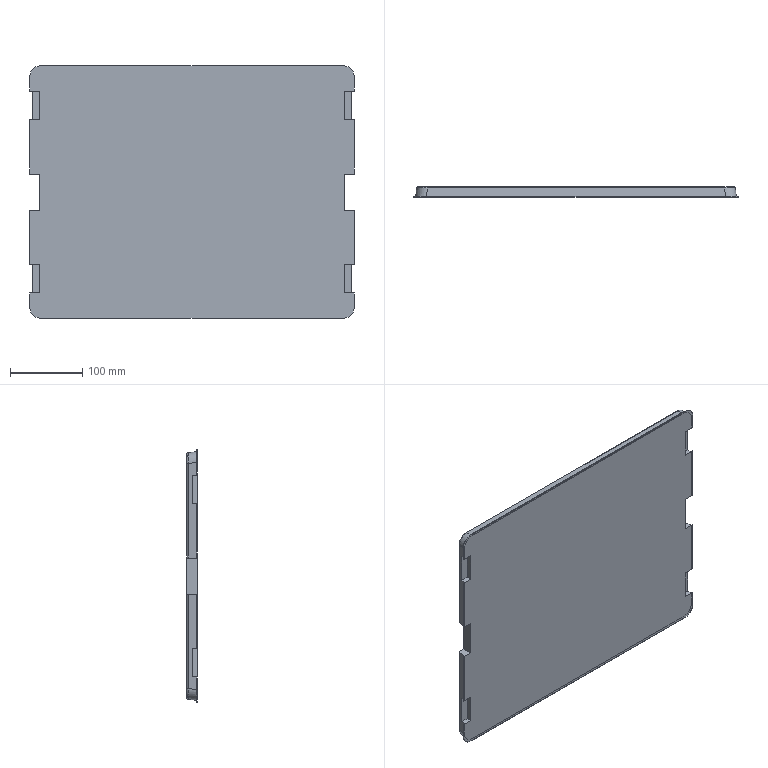Part | STEP file | 0246_Work-A | 1 solid | 68 faces | box 450 x 14 x 350 mm | volume 2100703 mm3 | plane 46 | cylinder 14 | spline 8 | commonest cylinder face diameters 30 x8 4 x6